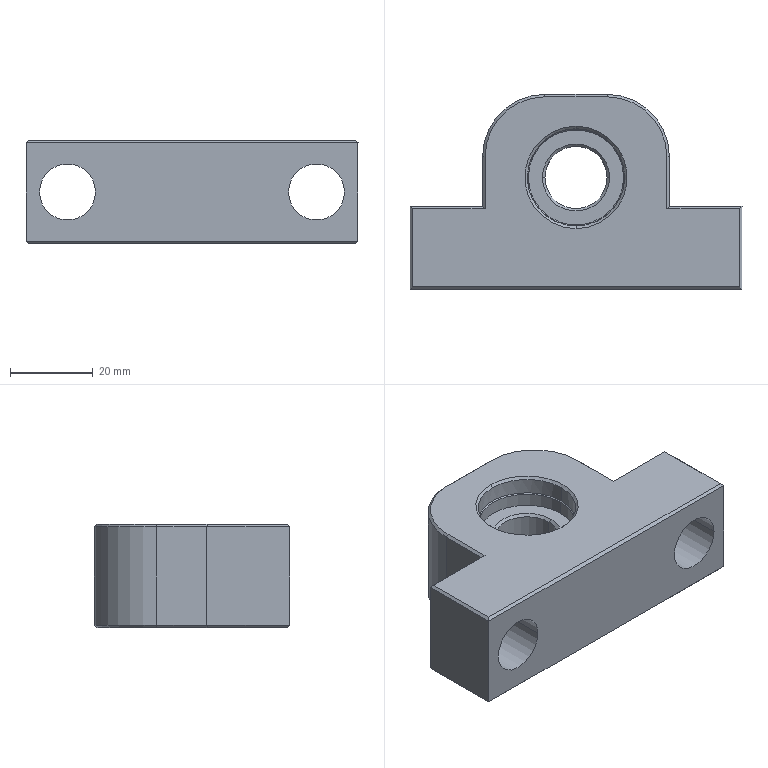Part | SolidWorks | features BaseBody 1 | 1 solid | 60 faces | box 80 x 47 x 25 mm | volume 53700 mm3 | plane 28 | cone 16 | cylinder 16 | commonest cylinder face diameters 13.5 x4 23 x4 23.5 x4 15 x2 30 x2